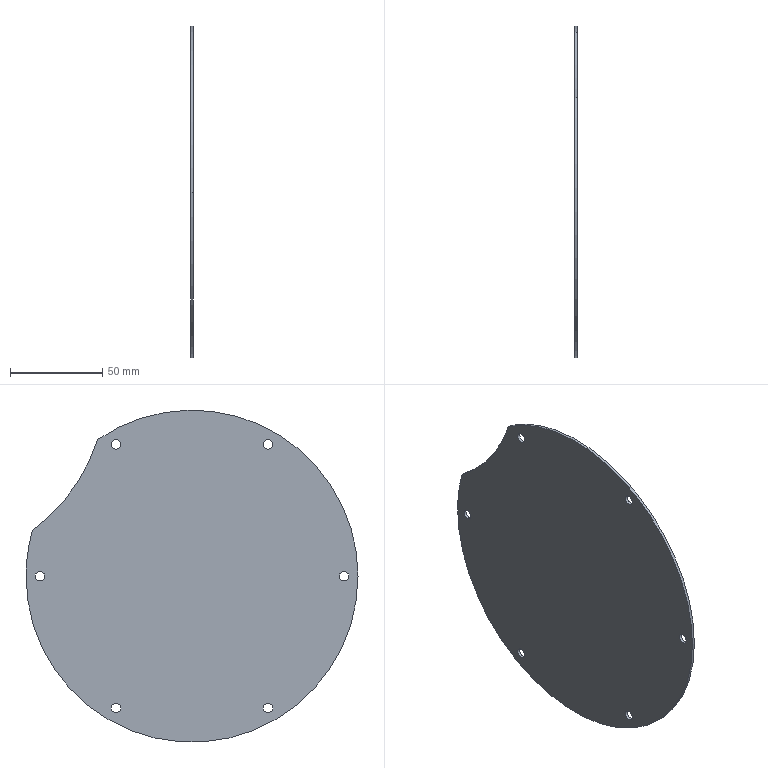Part | NX | features solid 2 | 1 solid | 18 faces | box 1.5 x 180 x 180 mm | volume 37369 mm3 | cylinder 16 | plane 2 | commonest cylinder face diameters 5.2 x12 180 x3 200 x1
STEP:
#1=CARTESIAN_POINT('',(-313.,-1086.102,330.));
#2=VERTEX_POINT('',#1);
#3=CARTESIAN_POINT('',(-311.5,-1086.102,330.));
#4=VERTEX_POINT('',#3);
#5=CARTESIAN_POINT('',(-58.437,-1086.102,330.));
#6=DIRECTION('',(-1.,0.,0.));
#7=VECTOR('',#6,1000.);
#8=LINE('',#5,#7);
#9=EDGE_CURVE('',#2,#4,#8,.F.);
#10=ORIENTED_EDGE('',*,*,#9,.T.);
#11=CARTESIAN_POINT('',(-311.5,-1091.302,330.));
#12=VERTEX_POINT('',#11);
#13=CARTESIAN_POINT('',(-311.5,-1088.702,330.));
#14=DIRECTION('',(-1.,0.,0.));
#15=DIRECTION('',(0.,-1.,0.));
#16=AXIS2_PLACEMENT_3D('',#13,#14,#15);
#17=CIRCLE('',#16,2.6);
#18=EDGE_CURVE('',#12,#4,#17,.T.);
#19=ORIENTED_EDGE('',*,*,#18,.F.);
#20=CARTESIAN_POINT('',(-313.,-1091.302,330.));
#21=VERTEX_POINT('',#20);
#22=CARTESIAN_POINT('',(-58.437,-1091.302,330.));
#23=DIRECTION('',(-1.,0.,0.));
#24=VECTOR('',#23,1000.);
#25=LINE('',#22,#24);
#26=EDGE_CURVE('',#12,#21,#25,.T.);
#27=ORIENTED_EDGE('',*,*,#26,.T.);
#28=CARTESIAN_POINT('',(-313.,-1088.702,330.));
#29=DIRECTION('',(-1.,0.,0.));
#30=DIRECTION('',(0.,-1.,0.));
#31=AXIS2_PLACEMENT_3D('',#28,#29,#30);
#32=CIRCLE('',#31,2.6);
#33=EDGE_CURVE('',#21,#2,#32,.T.);
#34=ORIENTED_EDGE('',*,*,#33,.T.);
#35=EDGE_LOOP('',(#10,#19,#27,#34));
#36=FACE_BOUND('',#35,.T.);
#37=CARTESIAN_POINT('',(-58.437,-1088.702,330.));
#38=DIRECTION('',(-1.,0.,0.));
#39=DIRECTION('',(0.,-1.,0.));
#40=AXIS2_PLACEMENT_3D('',#37,#38,#39);
#41=CYLINDRICAL_SURFACE('',#40,2.6);
#42=ADVANCED_FACE('',(#36),#41,.F.);
#43=CARTESIAN_POINT('',(-313.,-1127.352,258.553));
#44=VERTEX_POINT('',#43);
#45=CARTESIAN_POINT('',(-311.5,-1127.352,258.553));
#46=VERTEX_POINT('',#45);
#47=CARTESIAN_POINT('',(-58.437,-1127.352,258.553));
#48=DIRECTION('',(-1.,0.,0.));
#49=VECTOR('',#48,1000.);
#50=LINE('',#47,#49);
#51=EDGE_CURVE('',#44,#46,#50,.F.);
#52=ORIENTED_EDGE('',*,*,#51,.T.);
#53=CARTESIAN_POINT('',(-311.5,-1132.552,258.553));
#54=VERTEX_POINT('',#53);
#55=CARTESIAN_POINT('',(-311.5,-1129.952,258.553));
#56=DIRECTION('',(-1.,0.,0.));
#57=DIRECTION('',(0.,-1.,0.));
#58=AXIS2_PLACEMENT_3D('',#55,#56,#57);
#59=CIRCLE('',#58,2.6);
#60=EDGE_CURVE('',#54,#46,#59,.T.);
#61=ORIENTED_EDGE('',*,*,#60,.F.);
#62=CARTESIAN_POINT('',(-313.,-1132.552,258.553));
#63=VERTEX_POINT('',#62);
#64=CARTESIAN_POINT('',(-58.437,-1132.552,258.553));
#65=DIRECTION('',(-1.,0.,0.));
#66=VECTOR('',#65,1000.);
#67=LINE('',#64,#66);
#68=EDGE_CURVE('',#54,#63,#67,.T.);
#69=ORIENTED_EDGE('',*,*,#68,.T.);
#70=CARTESIAN_POINT('',(-313.,-1129.952,258.553));
#71=DIRECTION('',(-1.,0.,0.));
#72=DIRECTION('',(0.,-1.,0.));
#73=AXIS2_PLACEMENT_3D('',#70,#71,#72);
#74=CIRCLE('',#73,2.6);
#75=EDGE_CURVE('',#63,#44,#74,.T.);
#76=ORIENTED_EDGE('',*,*,#75,.T.);
#77=EDGE_LOOP('',(#52,#61,#69,#76));
#78=FACE_BOUND('',#77,.T.);
#79=CARTESIAN_POINT('',(-58.437,-1129.952,258.553));
#80=DIRECTION('',(-1.,0.,0.));
#81=DIRECTION('',(0.,-1.,0.));
#82=AXIS2_PLACEMENT_3D('',#79,#80,#81);
#83=CYLINDRICAL_SURFACE('',#82,2.6);
#84=ADVANCED_FACE('',(#78),#83,.F.);
#85=CARTESIAN_POINT('',(-313.,-1209.852,258.553));
#86=VERTEX_POINT('',#85);
#87=CARTESIAN_POINT('',(-311.5,-1209.852,258.553));
#88=VERTEX_POINT('',#87);
#89=CARTESIAN_POINT('',(-58.437,-1209.852,258.553));
#90=DIRECTION('',(-1.,0.,0.));
#91=VECTOR('',#90,1000.);
#92=LINE('',#89,#91);
#93=EDGE_CURVE('',#86,#88,#92,.F.);
#94=ORIENTED_EDGE('',*,*,#93,.T.);
#95=CARTESIAN_POINT('',(-311.5,-1215.052,258.553));
#96=VERTEX_POINT('',#95);
#97=CARTESIAN_POINT('',(-311.5,-1212.452,258.553));
#98=DIRECTION('',(-1.,0.,0.));
#99=DIRECTION('',(0.,-1.,0.));
#100=AXIS2_PLACEMENT_3D('',#97,#98,#99);
#101=CIRCLE('',#100,2.6);
#102=EDGE_CURVE('',#96,#88,#101,.T.);
#103=ORIENTED_EDGE('',*,*,#102,.F.);
#104=CARTESIAN_POINT('',(-313.,-1215.052,258.553));
#105=VERTEX_POINT('',#104);
#106=CARTESIAN_POINT('',(-58.437,-1215.052,258.553));
#107=DIRECTION('',(-1.,0.,0.));
#108=VECTOR('',#107,1000.);
#109=LINE('',#106,#108);
#110=EDGE_CURVE('',#96,#105,#109,.T.);
#111=ORIENTED_EDGE('',*,*,#110,.T.);
#112=CARTESIAN_POINT('',(-313.,-1212.452,258.553));
#113=DIRECTION('',(-1.,0.,0.));
#114=DIRECTION('',(0.,-1.,0.));
#115=AXIS2_PLACEMENT_3D('',#112,#113,#114);
#116=CIRCLE('',#115,2.6);
#117=EDGE_CURVE('',#105,#86,#116,.T.);
#118=ORIENTED_EDGE('',*,*,#117,.T.);
#119=EDGE_LOOP('',(#94,#103,#111,#118));
#120=FACE_BOUND('',#119,.T.);
#121=CARTESIAN_POINT('',(-58.437,-1212.452,258.553));
#122=DIRECTION('',(-1.,0.,0.));
#123=DIRECTION('',(0.,-1.,0.));
#124=AXIS2_PLACEMENT_3D('',#121,#122,#123);
#125=CYLINDRICAL_SURFACE('',#124,2.6);
#126=ADVANCED_FACE('',(#120),#125,.F.);
#127=CARTESIAN_POINT('',(-313.,-1251.102,330.));
#128=VERTEX_POINT('',#127);
#129=CARTESIAN_POINT('',(-311.5,-1251.102,330.));
#130=VERTEX_POINT('',#129);
#131=CARTESIAN_POINT('',(-58.437,-1251.102,330.));
#132=DIRECTION('',(-1.,0.,0.));
#133=VECTOR('',#132,1000.);
#134=LINE('',#131,#133);
#135=EDGE_CURVE('',#128,#130,#134,.F.);
#136=ORIENTED_EDGE('',*,*,#135,.T.);
#137=CARTESIAN_POINT('',(-311.5,-1256.302,330.));
#138=VERTEX_POINT('',#137);
#139=CARTESIAN_POINT('',(-311.5,-1253.702,330.));
#140=DIRECTION('',(-1.,0.,0.));
#141=DIRECTION('',(0.,-1.,0.));
#142=AXIS2_PLACEMENT_3D('',#139,#140,#141);
#143=CIRCLE('',#142,2.6);
#144=EDGE_CURVE('',#138,#130,#143,.T.);
#145=ORIENTED_EDGE('',*,*,#144,.F.);
#146=CARTESIAN_POINT('',(-313.,-1256.302,330.));
#147=VERTEX_POINT('',#146);
#148=CARTESIAN_POINT('',(-58.437,-1256.302,330.));
#149=DIRECTION('',(-1.,0.,0.));
#150=VECTOR('',#149,1000.);
#151=LINE('',#148,#150);
#152=EDGE_CURVE('',#138,#147,#151,.T.);
#153=ORIENTED_EDGE('',*,*,#152,.T.);
#154=CARTESIAN_POINT('',(-313.,-1253.702,330.));
#155=DIRECTION('',(-1.,0.,0.));
#156=DIRECTION('',(0.,-1.,0.));
#157=AXIS2_PLACEMENT_3D('',#154,#155,#156);
#158=CIRCLE('',#157,2.6);
#159=EDGE_CURVE('',#147,#128,#158,.T.);
#160=ORIENTED_EDGE('',*,*,#159,.T.);
#161=EDGE_LOOP('',(#136,#145,#153,#160));
#162=FACE_BOUND('',#161,.T.);
#163=CARTESIAN_POINT('',(-58.437,-1253.702,330.));
#164=DIRECTION('',(-1.,0.,0.));
#165=DIRECTION('',(0.,-1.,0.));
#166=AXIS2_PLACEMENT_3D('',#163,#164,#165);
#167=CYLINDRICAL_SURFACE('',#166,2.6);
#168=ADVANCED_FACE('',(#162),#167,.F.);
#169=CARTESIAN_POINT('',(-313.,-1209.852,401.447));
#170=VERTEX_POINT('',#169);
#171=CARTESIAN_POINT('',(-311.5,-1209.852,401.447));
#172=VERTEX_POINT('',#171);
#173=CARTESIAN_POINT('',(-58.437,-1209.852,401.447));
#174=DIRECTION('',(-1.,0.,0.));
#175=VECTOR('',#174,1000.);
#176=LINE('',#173,#175);
#177=EDGE_CURVE('',#170,#172,#176,.F.);
#178=ORIENTED_EDGE('',*,*,#177,.T.);
#179=CARTESIAN_POINT('',(-311.5,-1215.052,401.447));
#180=VERTEX_POINT('',#179);
#181=CARTESIAN_POINT('',(-311.5,-1212.452,401.447));
#182=DIRECTION('',(-1.,0.,0.));
#183=DIRECTION('',(0.,-1.,0.));
#184=AXIS2_PLACEMENT_3D('',#181,#182,#183);
#185=CIRCLE('',#184,2.6);
#186=EDGE_CURVE('',#180,#172,#185,.T.);
#187=ORIENTED_EDGE('',*,*,#186,.F.);
#188=CARTESIAN_POINT('',(-313.,-1215.052,401.447));
#189=VERTEX_POINT('',#188);
#190=CARTESIAN_POINT('',(-58.437,-1215.052,401.447));
#191=DIRECTION('',(-1.,0.,0.));
#192=VECTOR('',#191,1000.);
#193=LINE('',#190,#192);
#194=EDGE_CURVE('',#180,#189,#193,.T.);
#195=ORIENTED_EDGE('',*,*,#194,.T.);
#196=CARTESIAN_POINT('',(-313.,-1212.452,401.447));
#197=DIRECTION('',(-1.,0.,0.));
#198=DIRECTION('',(0.,-1.,0.));
#199=AXIS2_PLACEMENT_3D('',#196,#197,#198);
#200=CIRCLE('',#199,2.6);
#201=EDGE_CURVE('',#189,#170,#200,.T.);
#202=ORIENTED_EDGE('',*,*,#201,.T.);
#203=EDGE_LOOP('',(#178,#187,#195,#202));
#204=FACE_BOUND('',#203,.T.);
#205=CARTESIAN_POINT('',(-58.437,-1212.452,401.447));
#206=DIRECTION('',(-1.,0.,0.));
#207=DIRECTION('',(0.,-1.,0.));
#208=AXIS2_PLACEMENT_3D('',#205,#206,#207);
#209=CYLINDRICAL_SURFACE('',#208,2.6);
#210=ADVANCED_FACE('',(#204),#209,.F.);
#211=CARTESIAN_POINT('',(-311.5,-1127.352,401.447));
#212=VERTEX_POINT('',#211);
#213=CARTESIAN_POINT('',(-313.,-1127.352,401.447));
#214=VERTEX_POINT('',#213);
#215=CARTESIAN_POINT('',(-58.437,-1127.352,401.447));
#216=DIRECTION('',(-1.,0.,0.));
#217=VECTOR('',#216,1000.);
#218=LINE('',#215,#217);
#219=EDGE_CURVE('',#212,#214,#218,.T.);
#220=ORIENTED_EDGE('',*,*,#219,.F.);
#221=CARTESIAN_POINT('',(-311.5,-1132.552,401.447));
#222=VERTEX_POINT('',#221);
#223=CARTESIAN_POINT('',(-311.5,-1129.952,401.447));
#224=DIRECTION('',(-1.,0.,0.));
#225=DIRECTION('',(0.,-1.,0.));
#226=AXIS2_PLACEMENT_3D('',#223,#224,#225);
#227=CIRCLE('',#226,2.6);
#228=EDGE_CURVE('',#222,#212,#227,.T.);
#229=ORIENTED_EDGE('',*,*,#228,.F.);
#230=CARTESIAN_POINT('',(-313.,-1132.552,401.447));
#231=VERTEX_POINT('',#230);
#232=CARTESIAN_POINT('',(-58.437,-1132.552,401.447));
#233=DIRECTION('',(-1.,0.,0.));
#234=VECTOR('',#233,1000.);
#235=LINE('',#232,#234);
#236=EDGE_CURVE('',#231,#222,#235,.F.);
#237=ORIENTED_EDGE('',*,*,#236,.F.);
#238=CARTESIAN_POINT('',(-313.,-1129.952,401.447));
#239=DIRECTION('',(-1.,0.,0.));
#240=DIRECTION('',(0.,-1.,0.));
#241=AXIS2_PLACEMENT_3D('',#238,#239,#240);
#242=CIRCLE('',#241,2.6);
#243=EDGE_CURVE('',#231,#214,#242,.T.);
#244=ORIENTED_EDGE('',*,*,#243,.T.);
#245=EDGE_LOOP('',(#220,#229,#237,#244));
#246=FACE_BOUND('',#245,.T.);
#247=CARTESIAN_POINT('',(-58.437,-1129.952,401.447));
#248=DIRECTION('',(-1.,0.,0.));
#249=DIRECTION('',(0.,-1.,0.));
#250=AXIS2_PLACEMENT_3D('',#247,#248,#249);
#251=CYLINDRICAL_SURFACE('',#250,2.6);
#252=ADVANCED_FACE('',(#246),#251,.F.);
#253=ORIENTED_EDGE('',*,*,#243,.F.);
#254=CARTESIAN_POINT('',(-313.,-1129.952,401.447));
#255=DIRECTION('',(-1.,0.,0.));
#256=DIRECTION('',(0.,-1.,0.));
#257=AXIS2_PLACEMENT_3D('',#254,#255,#256);
#258=CIRCLE('',#257,2.6);
#259=EDGE_CURVE('',#214,#231,#258,.T.);
#260=ORIENTED_EDGE('',*,*,#259,.F.);
#261=EDGE_LOOP('',(#253,#260));
#262=FACE_BOUND('',#261,.T.);
#263=ORIENTED_EDGE('',*,*,#201,.F.);
#264=CARTESIAN_POINT('',(-313.,-1212.452,401.447));
#265=DIRECTION('',(-1.,0.,0.));
#266=DIRECTION('',(0.,-1.,0.));
#267=AXIS2_PLACEMENT_3D('',#264,#265,#266);
#268=CIRCLE('',#267,2.6);
#269=EDGE_CURVE('',#170,#189,#268,.T.);
#270=ORIENTED_EDGE('',*,*,#269,.F.);
#271=EDGE_LOOP('',(#263,#270));
#272=FACE_BOUND('',#271,.T.);
#273=ORIENTED_EDGE('',*,*,#159,.F.);
#274=CARTESIAN_POINT('',(-313.,-1253.702,330.));
#275=DIRECTION('',(-1.,0.,0.));
#276=DIRECTION('',(0.,-1.,0.));
#277=AXIS2_PLACEMENT_3D('',#274,#275,#276);
#278=CIRCLE('',#277,2.6);
#279=EDGE_CURVE('',#128,#147,#278,.T.);
#280=ORIENTED_EDGE('',*,*,#279,.F.);
#281=EDGE_LOOP('',(#273,#280));
#282=FACE_BOUND('',#281,.T.);
#283=ORIENTED_EDGE('',*,*,#117,.F.);
#284=CARTESIAN_POINT('',(-313.,-1212.452,258.553));
#285=DIRECTION('',(-1.,0.,0.));
#286=DIRECTION('',(0.,-1.,0.));
#287=AXIS2_PLACEMENT_3D('',#284,#285,#286);
#288=CIRCLE('',#287,2.6);
#289=EDGE_CURVE('',#86,#105,#288,.T.);
#290=ORIENTED_EDGE('',*,*,#289,.F.);
#291=EDGE_LOOP('',(#283,#290));
#292=FACE_BOUND('',#291,.T.);
#293=ORIENTED_EDGE('',*,*,#75,.F.);
#294=CARTESIAN_POINT('',(-313.,-1129.952,258.553));
#295=DIRECTION('',(-1.,0.,0.));
#296=DIRECTION('',(0.,-1.,0.));
#297=AXIS2_PLACEMENT_3D('',#294,#295,#296);
#298=CIRCLE('',#297,2.6);
#299=EDGE_CURVE('',#44,#63,#298,.T.);
#300=ORIENTED_EDGE('',*,*,#299,.F.);
#301=EDGE_LOOP('',(#293,#300));
#302=FACE_BOUND('',#301,.T.);
#303=ORIENTED_EDGE('',*,*,#33,.F.);
#304=CARTESIAN_POINT('',(-313.,-1088.702,330.));
#305=DIRECTION('',(-1.,0.,0.));
#306=DIRECTION('',(0.,-1.,0.));
#307=AXIS2_PLACEMENT_3D('',#304,#305,#306);
#308=CIRCLE('',#307,2.6);
#309=EDGE_CURVE('',#2,#21,#308,.T.);
#310=ORIENTED_EDGE('',*,*,#309,.F.);
#311=EDGE_LOOP('',(#303,#310));
#312=FACE_BOUND('',#311,.T.);
#313=CARTESIAN_POINT('',(-313.,-1084.674,354.756));
#314=VERTEX_POINT('',#313);
#315=CARTESIAN_POINT('',(-313.,-1120.102,404.086));
#316=VERTEX_POINT('',#315);
#317=CARTESIAN_POINT('',(-313.,-1025.,435.));
#318=DIRECTION('',(-1.,0.,0.));
#319=DIRECTION('',(0.,1.,0.));
#320=AXIS2_PLACEMENT_3D('',#317,#318,#319);
#321=CIRCLE('',#320,100.);
#322=EDGE_CURVE('',#314,#316,#321,.T.);
#323=ORIENTED_EDGE('',*,*,#322,.F.);
#324=CARTESIAN_POINT('',(-313.,-1081.202,330.));
#325=VERTEX_POINT('',#324);
#326=CARTESIAN_POINT('',(-313.,-1171.202,330.));
#327=DIRECTION('',(1.,0.,0.));
#328=DIRECTION('',(0.,0.,-1.));
#329=AXIS2_PLACEMENT_3D('',#326,#327,#328);
#330=CIRCLE('',#329,90.);
#331=EDGE_CURVE('',#325,#314,#330,.T.);
#332=ORIENTED_EDGE('',*,*,#331,.F.);
#333=CARTESIAN_POINT('',(-313.,-1261.202,330.));
#334=VERTEX_POINT('',#333);
#335=CARTESIAN_POINT('',(-313.,-1171.202,330.));
#336=DIRECTION('',(1.,0.,0.));
#337=DIRECTION('',(0.,0.,-1.));
#338=AXIS2_PLACEMENT_3D('',#335,#336,#337);
#339=CIRCLE('',#338,90.);
#340=EDGE_CURVE('',#334,#325,#339,.T.);
#341=ORIENTED_EDGE('',*,*,#340,.F.);
#342=CARTESIAN_POINT('',(-313.,-1171.202,330.));
#343=DIRECTION('',(1.,0.,0.));
#344=DIRECTION('',(0.,0.,-1.));
#345=AXIS2_PLACEMENT_3D('',#342,#343,#344);
#346=CIRCLE('',#345,90.);
#347=EDGE_CURVE('',#316,#334,#346,.T.);
#348=ORIENTED_EDGE('',*,*,#347,.F.);
#349=EDGE_LOOP('',(#323,#332,#341,#348));
#350=FACE_BOUND('',#349,.T.);
#351=CARTESIAN_POINT('',(-313.,-1098.101,382.5));
#352=DIRECTION('',(-1.,0.,0.));
#353=DIRECTION('',(0.,0.,1.));
#354=AXIS2_PLACEMENT_3D('',#351,#352,#353);
#355=PLANE('',#354);
#356=ADVANCED_FACE('',(#262,#272,#282,#292,#302,#312,#350),#355,.T.);
#357=ORIENTED_EDGE('',*,*,#228,.T.);
#358=CARTESIAN_POINT('',(-311.5,-1129.952,401.447));
#359=DIRECTION('',(-1.,0.,0.));
#360=DIRECTION('',(0.,-1.,0.));
#361=AXIS2_PLACEMENT_3D('',#358,#359,#360);
#362=CIRCLE('',#361,2.6);
#363=EDGE_CURVE('',#212,#222,#362,.T.);
#364=ORIENTED_EDGE('',*,*,#363,.T.);
#365=EDGE_LOOP('',(#357,#364));
#366=FACE_BOUND('',#365,.T.);
#367=ORIENTED_EDGE('',*,*,#186,.T.);
#368=CARTESIAN_POINT('',(-311.5,-1212.452,401.447));
#369=DIRECTION('',(-1.,0.,0.));
#370=DIRECTION('',(0.,-1.,0.));
#371=AXIS2_PLACEMENT_3D('',#368,#369,#370);
#372=CIRCLE('',#371,2.6);
#373=EDGE_CURVE('',#172,#180,#372,.T.);
#374=ORIENTED_EDGE('',*,*,#373,.T.);
#375=EDGE_LOOP('',(#367,#374));
#376=FACE_BOUND('',#375,.T.);
#377=ORIENTED_EDGE('',*,*,#144,.T.);
#378=CARTESIAN_POINT('',(-311.5,-1253.702,330.));
#379=DIRECTION('',(-1.,0.,0.));
#380=DIRECTION('',(0.,-1.,0.));
#381=AXIS2_PLACEMENT_3D('',#378,#379,#380);
#382=CIRCLE('',#381,2.6);
#383=EDGE_CURVE('',#130,#138,#382,.T.);
#384=ORIENTED_EDGE('',*,*,#383,.T.);
#385=EDGE_LOOP('',(#377,#384));
#386=FACE_BOUND('',#385,.T.);
#387=ORIENTED_EDGE('',*,*,#102,.T.);
#388=CARTESIAN_POINT('',(-311.5,-1212.452,258.553));
#389=DIRECTION('',(-1.,0.,0.));
#390=DIRECTION('',(0.,-1.,0.));
#391=AXIS2_PLACEMENT_3D('',#388,#389,#390);
#392=CIRCLE('',#391,2.6);
#393=EDGE_CURVE('',#88,#96,#392,.T.);
#394=ORIENTED_EDGE('',*,*,#393,.T.);
#395=EDGE_LOOP('',(#387,#394));
#396=FACE_BOUND('',#395,.T.);
#397=ORIENTED_EDGE('',*,*,#60,.T.);
#398=CARTESIAN_POINT('',(-311.5,-1129.952,258.553));
#399=DIRECTION('',(-1.,0.,0.));
#400=DIRECTION('',(0.,-1.,0.));
#401=AXIS2_PLACEMENT_3D('',#398,#399,#400);
#402=CIRCLE('',#401,2.6);
#403=EDGE_CURVE('',#46,#54,#402,.T.);
#404=ORIENTED_EDGE('',*,*,#403,.T.);
#405=EDGE_LOOP('',(#397,#404));
#406=FACE_BOUND('',#405,.T.);
#407=ORIENTED_EDGE('',*,*,#18,.T.);
#408=CARTESIAN_POINT('',(-311.5,-1088.702,330.));
#409=DIRECTION('',(-1.,0.,0.));
#410=DIRECTION('',(0.,-1.,0.));
#411=AXIS2_PLACEMENT_3D('',#408,#409,#410);
#412=CIRCLE('',#411,2.6);
#413=EDGE_CURVE('',#4,#12,#412,.T.);
#414=ORIENTED_EDGE('',*,*,#413,.T.);
#415=EDGE_LOOP('',(#407,#414));
#416=FACE_BOUND('',#415,.T.);
#417=CARTESIAN_POINT('',(-311.5,-1084.674,354.756));
#418=VERTEX_POINT('',#417);
#419=CARTESIAN_POINT('',(-311.5,-1120.102,404.086));
#420=VERTEX_POINT('',#419);
#421=CARTESIAN_POINT('',(-311.5,-1025.,435.));
#422=DIRECTION('',(-1.,0.,0.));
#423=DIRECTION('',(0.,1.,0.));
#424=AXIS2_PLACEMENT_3D('',#421,#422,#423);
#425=CIRCLE('',#424,100.);
#426=EDGE_CURVE('',#418,#420,#425,.T.);
#427=ORIENTED_EDGE('',*,*,#426,.T.);
#428=CARTESIAN_POINT('',(-311.5,-1261.202,330.));
#429=VERTEX_POINT('',#428);
#430=CARTESIAN_POINT('',(-311.5,-1171.202,330.));
#431=DIRECTION('',(1.,0.,0.));
#432=DIRECTION('',(0.,0.,-1.));
#433=AXIS2_PLACEMENT_3D('',#430,#431,#432);
#434=CIRCLE('',#433,90.);
#435=EDGE_CURVE('',#420,#429,#434,.T.);
#436=ORIENTED_EDGE('',*,*,#435,.T.);
#437=CARTESIAN_POINT('',(-311.5,-1081.202,330.));
#438=VERTEX_POINT('',#437);
#439=CARTESIAN_POINT('',(-311.5,-1171.202,330.));
#440=DIRECTION('',(1.,0.,0.));
#441=DIRECTION('',(0.,0.,-1.));
#442=AXIS2_PLACEMENT_3D('',#439,#440,#441);
#443=CIRCLE('',#442,90.);
#444=EDGE_CURVE('',#429,#438,#443,.T.);
#445=ORIENTED_EDGE('',*,*,#444,.T.);
#446=CARTESIAN_POINT('',(-311.5,-1171.202,330.));
#447=DIRECTION('',(1.,0.,0.));
#448=DIRECTION('',(0.,0.,-1.));
#449=AXIS2_PLACEMENT_3D('',#446,#447,#448);
#450=CIRCLE('',#449,90.);
#451=EDGE_CURVE('',#438,#418,#450,.T.);
#452=ORIENTED_EDGE('',*,*,#451,.T.);
#453=EDGE_LOOP('',(#427,#436,#445,#452));
#454=FACE_BOUND('',#453,.T.);
#455=CARTESIAN_POINT('',(-311.5,-1098.101,382.5));
#456=DIRECTION('',(-1.,0.,0.));
#457=DIRECTION('',(0.,0.,1.));
#458=AXIS2_PLACEMENT_3D('',#455,#456,#457);
#459=PLANE('',#458);
#460=ADVANCED_FACE('',(#366,#376,#386,#396,#406,#416,#454),#459,.F.);
#461=CARTESIAN_POINT('',(-311.5,-1261.202,330.));
#462=DIRECTION('',(-1.,0.,0.));
#463=VECTOR('',#462,1000.);
#464=LINE('',#461,#463);
#465=EDGE_CURVE('',#429,#334,#464,.T.);
#466=ORIENTED_EDGE('',*,*,#465,.F.);
#467=ORIENTED_EDGE('',*,*,#435,.F.);
#468=CARTESIAN_POINT('',(-311.5,-1120.102,404.086));
#469=DIRECTION('',(-1.,0.,0.));
#470=VECTOR('',#469,1000.);
#471=LINE('',#468,#470);
#472=EDGE_CURVE('',#420,#316,#471,.T.);
#473=ORIENTED_EDGE('',*,*,#472,.T.);
#474=ORIENTED_EDGE('',*,*,#347,.T.);
#475=EDGE_LOOP('',(#466,#467,#473,#474));
#476=FACE_BOUND('',#475,.T.);
#477=CARTESIAN_POINT('',(-311.5,-1171.202,330.));
#478=DIRECTION('',(-1.,0.,0.));
#479=DIRECTION('',(0.,-1.,0.));
#480=AXIS2_PLACEMENT_3D('',#477,#478,#479);
#481=CYLINDRICAL_SURFACE('',#480,90.);
#482=ADVANCED_FACE('',(#476),#481,.T.);
#483=ORIENTED_EDGE('',*,*,#322,.T.);
#484=ORIENTED_EDGE('',*,*,#472,.F.);
#485=ORIENTED_EDGE('',*,*,#426,.F.);
#486=CARTESIAN_POINT('',(-311.5,-1084.674,354.756));
#487=DIRECTION('',(-1.,0.,0.));
#488=VECTOR('',#487,1000.);
#489=LINE('',#486,#488);
#490=EDGE_CURVE('',#418,#314,#489,.T.);
#491=ORIENTED_EDGE('',*,*,#490,.T.);
#492=EDGE_LOOP('',(#483,#484,#485,#491));
#493=FACE_BOUND('',#492,.T.);
#494=CARTESIAN_POINT('',(-311.5,-1025.,435.));
#495=DIRECTION('',(-1.,0.,0.));
#496=DIRECTION('',(0.,-1.,0.));
#497=AXIS2_PLACEMENT_3D('',#494,#495,#496);
#498=CYLINDRICAL_SURFACE('',#497,100.);
#499=ADVANCED_FACE('',(#493),#498,.F.);
#500=CARTESIAN_POINT('',(-311.5,-1081.202,330.));
#501=DIRECTION('',(-1.,0.,0.));
#502=VECTOR('',#501,1000.);
#503=LINE('',#500,#502);
#504=EDGE_CURVE('',#438,#325,#503,.T.);
#505=ORIENTED_EDGE('',*,*,#504,.F.);
#506=ORIENTED_EDGE('',*,*,#444,.F.);
#507=ORIENTED_EDGE('',*,*,#465,.T.);
#508=ORIENTED_EDGE('',*,*,#340,.T.);
#509=EDGE_LOOP('',(#505,#506,#507,#508));
#510=FACE_BOUND('',#509,.T.);
#511=CARTESIAN_POINT('',(-311.5,-1171.202,330.));
#512=DIRECTION('',(-1.,0.,0.));
#513=DIRECTION('',(0.,-1.,0.));
#514=AXIS2_PLACEMENT_3D('',#511,#512,#513);
#515=CYLINDRICAL_SURFACE('',#514,90.);
#516=ADVANCED_FACE('',(#510),#515,.T.);
#517=ORIENTED_EDGE('',*,*,#451,.F.);
#518=ORIENTED_EDGE('',*,*,#504,.T.);
#519=ORIENTED_EDGE('',*,*,#331,.T.);
#520=ORIENTED_EDGE('',*,*,#490,.F.);
#521=EDGE_LOOP('',(#517,#518,#519,#520));
#522=FACE_BOUND('',#521,.T.);
#523=CARTESIAN_POINT('',(-311.5,-1171.202,330.));
#524=DIRECTION('',(-1.,0.,0.));
#525=DIRECTION('',(0.,-1.,0.));
#526=AXIS2_PLACEMENT_3D('',#523,#524,#525);
#527=CYLINDRICAL_SURFACE('',#526,90.);
#528=ADVANCED_FACE('',(#522),#527,.T.);
#529=ORIENTED_EDGE('',*,*,#363,.F.);
#530=ORIENTED_EDGE('',*,*,#219,.T.);
#531=ORIENTED_EDGE('',*,*,#259,.T.);
#532=ORIENTED_EDGE('',*,*,#236,.T.);
#533=EDGE_LOOP('',(#529,#530,#531,#532));
#534=FACE_BOUND('',#533,.T.);
#535=CARTESIAN_POINT('',(-58.437,-1129.952,401.447));
#536=DIRECTION('',(-1.,0.,0.));
#537=DIRECTION('',(0.,-1.,0.));
#538=AXIS2_PLACEMENT_3D('',#535,#536,#537);
#539=CYLINDRICAL_SURFACE('',#538,2.6);
#540=ADVANCED_FACE('',(#534),#539,.F.);
#541=ORIENTED_EDGE('',*,*,#373,.F.);
#542=ORIENTED_EDGE('',*,*,#177,.F.);
#543=ORIENTED_EDGE('',*,*,#269,.T.);
#544=ORIENTED_EDGE('',*,*,#194,.F.);
#545=EDGE_LOOP('',(#541,#542,#543,#544));
#546=FACE_BOUND('',#545,.T.);
#547=CARTESIAN_POINT('',(-58.437,-1212.452,401.447));
#548=DIRECTION('',(-1.,0.,0.));
#549=DIRECTION('',(0.,-1.,0.));
#550=AXIS2_PLACEMENT_3D('',#547,#548,#549);
#551=CYLINDRICAL_SURFACE('',#550,2.6);
#552=ADVANCED_FACE('',(#546),#551,.F.);
#553=ORIENTED_EDGE('',*,*,#383,.F.);
#554=ORIENTED_EDGE('',*,*,#135,.F.);
#555=ORIENTED_EDGE('',*,*,#279,.T.);
#556=ORIENTED_EDGE('',*,*,#152,.F.);
#557=EDGE_LOOP('',(#553,#554,#555,#556));
#558=FACE_BOUND('',#557,.T.);
#559=CARTESIAN_POINT('',(-58.437,-1253.702,330.));
#560=DIRECTION('',(-1.,0.,0.));
#561=DIRECTION('',(0.,-1.,0.));
#562=AXIS2_PLACEMENT_3D('',#559,#560,#561);
#563=CYLINDRICAL_SURFACE('',#562,2.6);
#564=ADVANCED_FACE('',(#558),#563,.F.);
#565=ORIENTED_EDGE('',*,*,#393,.F.);
#566=ORIENTED_EDGE('',*,*,#93,.F.);
#567=ORIENTED_EDGE('',*,*,#289,.T.);
#568=ORIENTED_EDGE('',*,*,#110,.F.);
#569=EDGE_LOOP('',(#565,#566,#567,#568));
#570=FACE_BOUND('',#569,.T.);
#571=CARTESIAN_POINT('',(-58.437,-1212.452,258.553));
#572=DIRECTION('',(-1.,0.,0.));
#573=DIRECTION('',(0.,-1.,0.));
#574=AXIS2_PLACEMENT_3D('',#571,#572,#573);
#575=CYLINDRICAL_SURFACE('',#574,2.6);
#576=ADVANCED_FACE('',(#570),#575,.F.);
#577=ORIENTED_EDGE('',*,*,#403,.F.);
#578=ORIENTED_EDGE('',*,*,#51,.F.);
#579=ORIENTED_EDGE('',*,*,#299,.T.);
#580=ORIENTED_EDGE('',*,*,#68,.F.);
#581=EDGE_LOOP('',(#577,#578,#579,#580));
#582=FACE_BOUND('',#581,.T.);
#583=CARTESIAN_POINT('',(-58.437,-1129.952,258.553));
#584=DIRECTION('',(-1.,0.,0.));
#585=DIRECTION('',(0.,-1.,0.));
#586=AXIS2_PLACEMENT_3D('',#583,#584,#585);
#587=CYLINDRICAL_SURFACE('',#586,2.6);
#588=ADVANCED_FACE('',(#582),#587,.F.);
#589=ORIENTED_EDGE('',*,*,#413,.F.);
#590=ORIENTED_EDGE('',*,*,#9,.F.);
#591=ORIENTED_EDGE('',*,*,#309,.T.);
#592=ORIENTED_EDGE('',*,*,#26,.F.);
#593=EDGE_LOOP('',(#589,#590,#591,#592));
#594=FACE_BOUND('',#593,.T.);
#595=CARTESIAN_POINT('',(-58.437,-1088.702,330.));
#596=DIRECTION('',(-1.,0.,0.));
#597=DIRECTION('',(0.,-1.,0.));
#598=AXIS2_PLACEMENT_3D('',#595,#596,#597);
#599=CYLINDRICAL_SURFACE('',#598,2.6);
#600=ADVANCED_FACE('',(#594),#599,.F.);
#601=CLOSED_SHELL('',(#42,#84,#126,#168,#210,#252,#356,#460,#482,#499,#516,#528,#540,#552,#564,#576,#588,#600));
#602=MANIFOLD_SOLID_BREP('',#601);
#603=(LENGTH_UNIT()NAMED_UNIT(*)SI_UNIT(.MILLI.,.METRE.));
#604=UNCERTAINTY_MEASURE_WITH_UNIT(LENGTH_MEASURE(0.00001),#603,'','');
#605=(NAMED_UNIT(*)PLANE_ANGLE_UNIT()SI_UNIT($,.RADIAN.));
#606=(NAMED_UNIT(*)SI_UNIT($,.STERADIAN.)SOLID_ANGLE_UNIT());
#607=(GEOMETRIC_REPRESENTATION_CONTEXT(3)GLOBAL_UNCERTAINTY_ASSIGNED_CONTEXT((#604))GLOBAL_UNIT_ASSIGNED_CONTEXT((#603,#605,#606))REPRESENTATION_CONTEXT('',''));
#608=ADVANCED_BREP_SHAPE_REPRESENTATION('',(#602),#607);